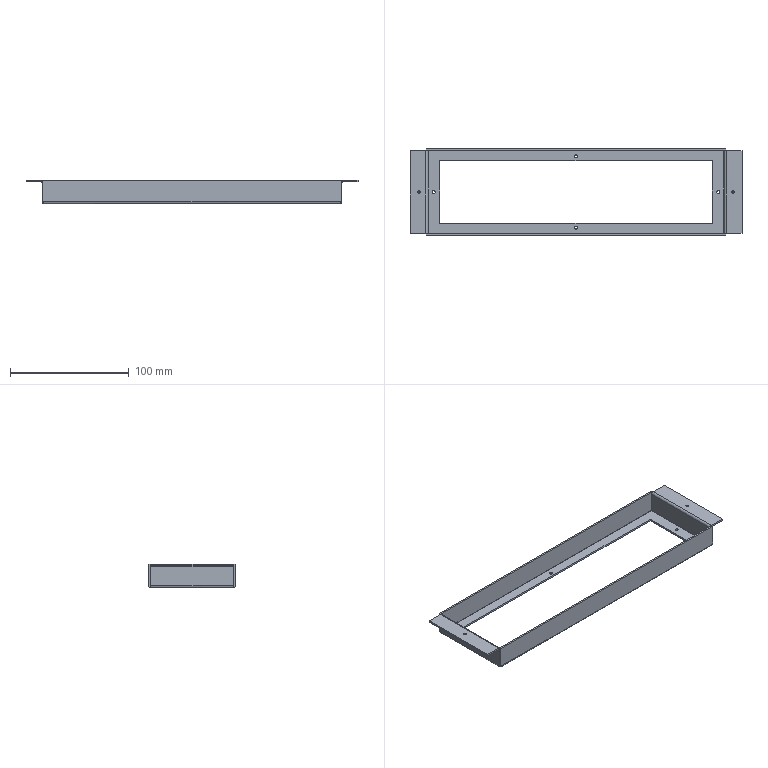Part | STEP file | FHD-021-001-Q rack welded part Q | 1 solid | 72 faces | box 280 x 73 x 20 mm | volume 29608 mm3 | plane 46 | cylinder 18 | spline 8 | commonest cylinder face diameters 0.4 x6 3.4 x6 2.5 x4 2 x2